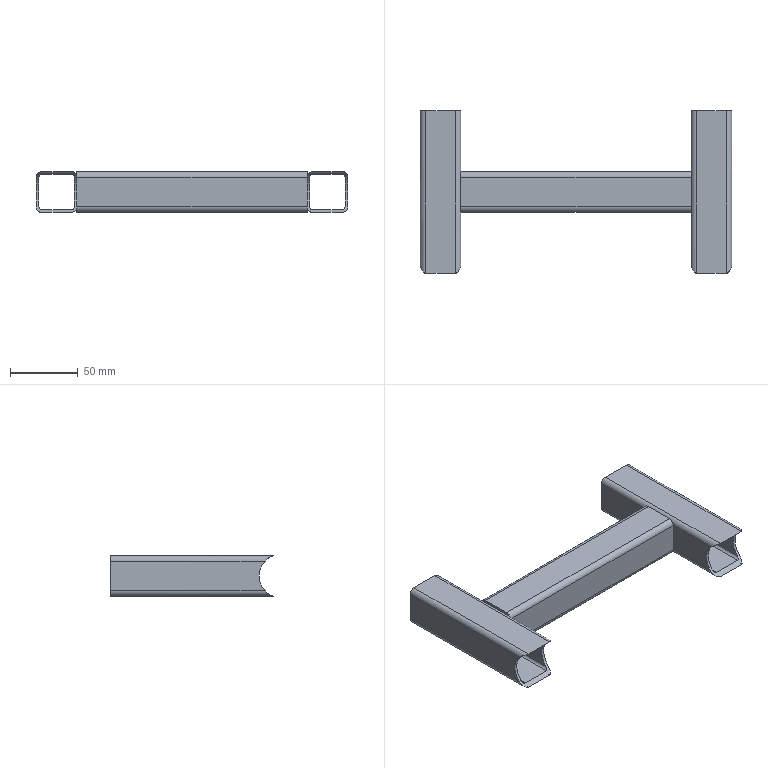Part | SolidWorks | features ICE 1, WeldMemberFeat 1, WeldmentFeature 1 | 3 solids | 54 faces | box 230 x 120 x 30 mm | volume 85383 mm3 | plane 28 | cylinder 26 | commonest cylinder face diameters 4 x12 8 x12 32 x2